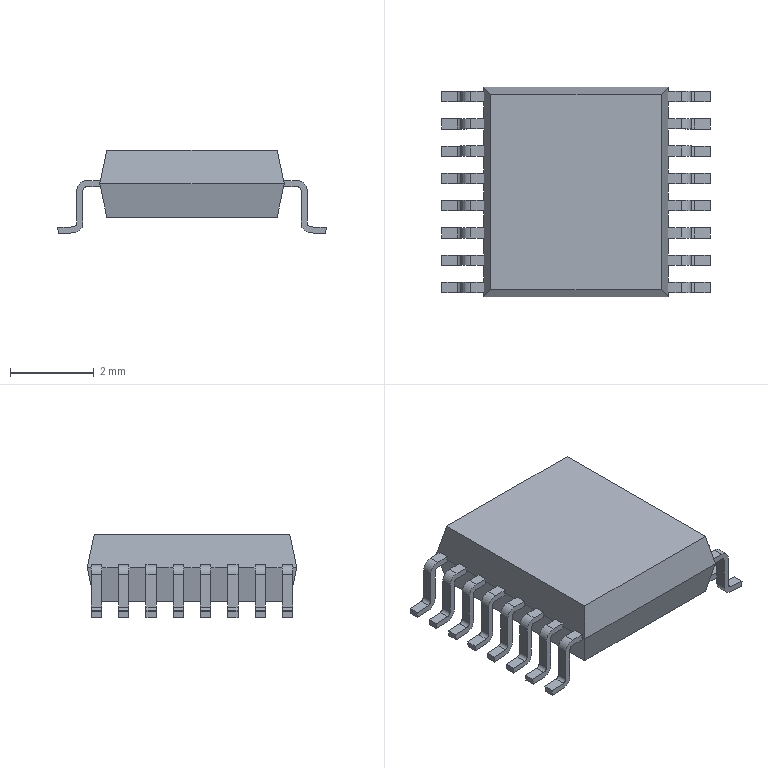Part | STEP file | RJ-USIO-V1_2-220411_287 | 1 solid | 218 faces | box 6.4 x 5 x 2 mm | volume 33.822 mm3 | plane 154 | cylinder 64 | commonest cylinder face diameters 0.18 x32 0.47 x32